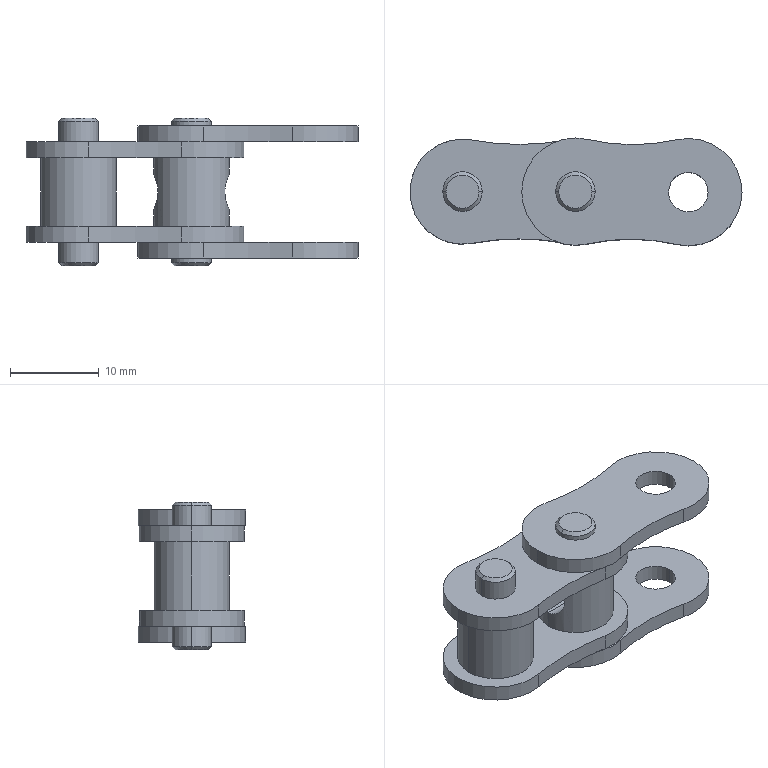Part | STEP file | 3 solids | 62 faces | box 37.34 x 12.127 x 16.625 mm | volume 2631 mm3 | cylinder 42 | plane 12 | cone 8 | commonest cylinder face diameters 4.45 x16 11.81 x6 12.07 x6 8.51 x4 44.615 x4 57.066 x4